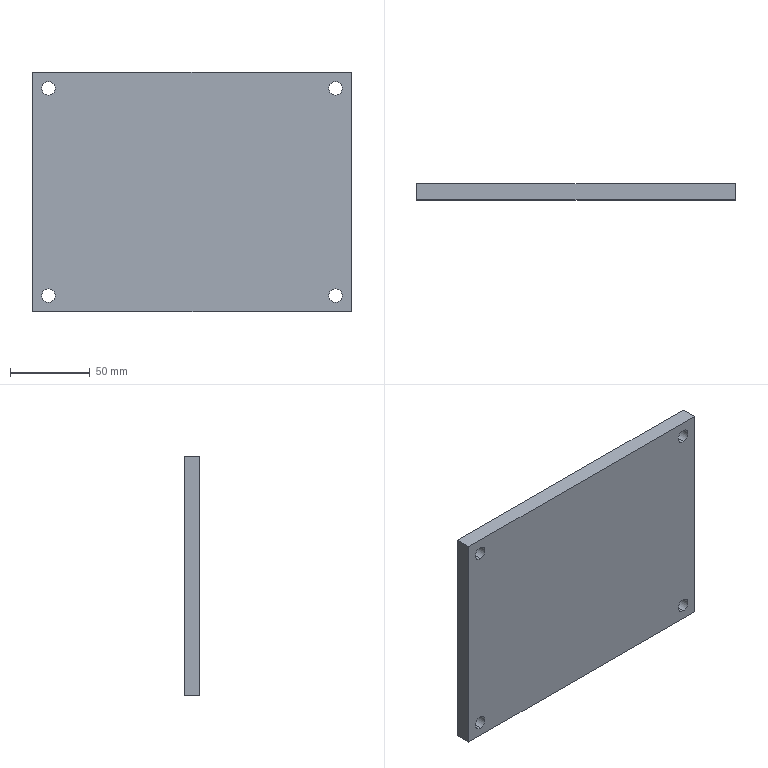Part | 1 solid | 14 faces | box 200 x 10 x 150 mm | volume 297730 mm3 | cylinder 8 | plane 6 | commonest cylinder face diameters 8.5 x8
STEP:
#1=CARTESIAN_POINT('',(-90.,10.,69.25));
#2=VERTEX_POINT('',#1);
#3=CARTESIAN_POINT('',(-90.,10.,60.75));
#4=VERTEX_POINT('',#3);
#5=CARTESIAN_POINT('',(-90.,10.,65.));
#6=DIRECTION('',(0.,-1.,0.));
#7=DIRECTION('',(0.,0.,-1.));
#8=AXIS2_PLACEMENT_3D('',#5,#6,#7);
#9=CIRCLE('',#8,4.25);
#10=EDGE_CURVE('',#2,#4,#9,.T.);
#11=ORIENTED_EDGE('',*,*,#10,.F.);
#12=CARTESIAN_POINT('',(-90.,0.,69.25));
#13=VERTEX_POINT('',#12);
#14=CARTESIAN_POINT('',(-90.,0.,69.25));
#15=DIRECTION('',(0.,-1.,0.));
#16=VECTOR('',#15,1000.);
#17=LINE('',#14,#16);
#18=EDGE_CURVE('',#2,#13,#17,.T.);
#19=ORIENTED_EDGE('',*,*,#18,.T.);
#20=CARTESIAN_POINT('',(-90.,0.,60.75));
#21=VERTEX_POINT('',#20);
#22=CARTESIAN_POINT('',(-90.,0.,65.));
#23=DIRECTION('',(0.,-1.,0.));
#24=DIRECTION('',(0.,0.,-1.));
#25=AXIS2_PLACEMENT_3D('',#22,#23,#24);
#26=CIRCLE('',#25,4.25);
#27=EDGE_CURVE('',#13,#21,#26,.T.);
#28=ORIENTED_EDGE('',*,*,#27,.T.);
#29=CARTESIAN_POINT('',(-90.,0.,60.75));
#30=DIRECTION('',(0.,-1.,0.));
#31=VECTOR('',#30,1000.);
#32=LINE('',#29,#31);
#33=EDGE_CURVE('',#4,#21,#32,.T.);
#34=ORIENTED_EDGE('',*,*,#33,.F.);
#35=EDGE_LOOP('',(#11,#19,#28,#34));
#36=FACE_OUTER_BOUND('',#35,.T.);
#37=CARTESIAN_POINT('',(-90.,0.,65.));
#38=DIRECTION('',(0.,-1.,0.));
#39=DIRECTION('',(0.,0.,-1.));
#40=AXIS2_PLACEMENT_3D('',#37,#38,#39);
#41=CYLINDRICAL_SURFACE('',#40,4.25);
#42=ADVANCED_FACE('',(#36),#41,.F.);
#43=CARTESIAN_POINT('',(-90.,10.,-60.75));
#44=VERTEX_POINT('',#43);
#45=CARTESIAN_POINT('',(-90.,10.,-69.25));
#46=VERTEX_POINT('',#45);
#47=CARTESIAN_POINT('',(-90.,10.,-65.));
#48=DIRECTION('',(0.,-1.,0.));
#49=DIRECTION('',(0.,0.,-1.));
#50=AXIS2_PLACEMENT_3D('',#47,#48,#49);
#51=CIRCLE('',#50,4.25);
#52=EDGE_CURVE('',#44,#46,#51,.T.);
#53=ORIENTED_EDGE('',*,*,#52,.F.);
#54=CARTESIAN_POINT('',(-90.,0.,-60.75));
#55=VERTEX_POINT('',#54);
#56=CARTESIAN_POINT('',(-90.,0.,-60.75));
#57=DIRECTION('',(0.,-1.,0.));
#58=VECTOR('',#57,1000.);
#59=LINE('',#56,#58);
#60=EDGE_CURVE('',#44,#55,#59,.T.);
#61=ORIENTED_EDGE('',*,*,#60,.T.);
#62=CARTESIAN_POINT('',(-90.,0.,-69.25));
#63=VERTEX_POINT('',#62);
#64=CARTESIAN_POINT('',(-90.,0.,-65.));
#65=DIRECTION('',(0.,-1.,0.));
#66=DIRECTION('',(0.,0.,-1.));
#67=AXIS2_PLACEMENT_3D('',#64,#65,#66);
#68=CIRCLE('',#67,4.25);
#69=EDGE_CURVE('',#55,#63,#68,.T.);
#70=ORIENTED_EDGE('',*,*,#69,.T.);
#71=CARTESIAN_POINT('',(-90.,0.,-69.25));
#72=DIRECTION('',(0.,-1.,0.));
#73=VECTOR('',#72,1000.);
#74=LINE('',#71,#73);
#75=EDGE_CURVE('',#46,#63,#74,.T.);
#76=ORIENTED_EDGE('',*,*,#75,.F.);
#77=EDGE_LOOP('',(#53,#61,#70,#76));
#78=FACE_OUTER_BOUND('',#77,.T.);
#79=CARTESIAN_POINT('',(-90.,0.,-65.));
#80=DIRECTION('',(0.,-1.,0.));
#81=DIRECTION('',(0.,0.,-1.));
#82=AXIS2_PLACEMENT_3D('',#79,#80,#81);
#83=CYLINDRICAL_SURFACE('',#82,4.25);
#84=ADVANCED_FACE('',(#78),#83,.F.);
#85=CARTESIAN_POINT('',(90.,10.,-60.75));
#86=VERTEX_POINT('',#85);
#87=CARTESIAN_POINT('',(90.,10.,-69.25));
#88=VERTEX_POINT('',#87);
#89=CARTESIAN_POINT('',(90.,10.,-65.));
#90=DIRECTION('',(0.,-1.,0.));
#91=DIRECTION('',(0.,0.,-1.));
#92=AXIS2_PLACEMENT_3D('',#89,#90,#91);
#93=CIRCLE('',#92,4.25);
#94=EDGE_CURVE('',#86,#88,#93,.T.);
#95=ORIENTED_EDGE('',*,*,#94,.F.);
#96=CARTESIAN_POINT('',(90.,0.,-60.75));
#97=VERTEX_POINT('',#96);
#98=CARTESIAN_POINT('',(90.,0.,-60.75));
#99=DIRECTION('',(0.,-1.,0.));
#100=VECTOR('',#99,1000.);
#101=LINE('',#98,#100);
#102=EDGE_CURVE('',#86,#97,#101,.T.);
#103=ORIENTED_EDGE('',*,*,#102,.T.);
#104=CARTESIAN_POINT('',(90.,0.,-69.25));
#105=VERTEX_POINT('',#104);
#106=CARTESIAN_POINT('',(90.,0.,-65.));
#107=DIRECTION('',(0.,-1.,0.));
#108=DIRECTION('',(0.,0.,-1.));
#109=AXIS2_PLACEMENT_3D('',#106,#107,#108);
#110=CIRCLE('',#109,4.25);
#111=EDGE_CURVE('',#97,#105,#110,.T.);
#112=ORIENTED_EDGE('',*,*,#111,.T.);
#113=CARTESIAN_POINT('',(90.,0.,-69.25));
#114=DIRECTION('',(0.,-1.,0.));
#115=VECTOR('',#114,1000.);
#116=LINE('',#113,#115);
#117=EDGE_CURVE('',#88,#105,#116,.T.);
#118=ORIENTED_EDGE('',*,*,#117,.F.);
#119=EDGE_LOOP('',(#95,#103,#112,#118));
#120=FACE_OUTER_BOUND('',#119,.T.);
#121=CARTESIAN_POINT('',(90.,0.,-65.));
#122=DIRECTION('',(0.,-1.,0.));
#123=DIRECTION('',(0.,0.,-1.));
#124=AXIS2_PLACEMENT_3D('',#121,#122,#123);
#125=CYLINDRICAL_SURFACE('',#124,4.25);
#126=ADVANCED_FACE('',(#120),#125,.F.);
#127=CARTESIAN_POINT('',(90.,10.,69.25));
#128=VERTEX_POINT('',#127);
#129=CARTESIAN_POINT('',(90.,10.,60.75));
#130=VERTEX_POINT('',#129);
#131=CARTESIAN_POINT('',(90.,10.,65.));
#132=DIRECTION('',(0.,-1.,0.));
#133=DIRECTION('',(0.,0.,-1.));
#134=AXIS2_PLACEMENT_3D('',#131,#132,#133);
#135=CIRCLE('',#134,4.25);
#136=EDGE_CURVE('',#128,#130,#135,.T.);
#137=ORIENTED_EDGE('',*,*,#136,.F.);
#138=CARTESIAN_POINT('',(90.,0.,69.25));
#139=VERTEX_POINT('',#138);
#140=CARTESIAN_POINT('',(90.,0.,69.25));
#141=DIRECTION('',(0.,-1.,0.));
#142=VECTOR('',#141,1000.);
#143=LINE('',#140,#142);
#144=EDGE_CURVE('',#128,#139,#143,.T.);
#145=ORIENTED_EDGE('',*,*,#144,.T.);
#146=CARTESIAN_POINT('',(90.,0.,60.75));
#147=VERTEX_POINT('',#146);
#148=CARTESIAN_POINT('',(90.,0.,65.));
#149=DIRECTION('',(0.,-1.,0.));
#150=DIRECTION('',(0.,0.,-1.));
#151=AXIS2_PLACEMENT_3D('',#148,#149,#150);
#152=CIRCLE('',#151,4.25);
#153=EDGE_CURVE('',#139,#147,#152,.T.);
#154=ORIENTED_EDGE('',*,*,#153,.T.);
#155=CARTESIAN_POINT('',(90.,0.,60.75));
#156=DIRECTION('',(0.,-1.,0.));
#157=VECTOR('',#156,1000.);
#158=LINE('',#155,#157);
#159=EDGE_CURVE('',#130,#147,#158,.T.);
#160=ORIENTED_EDGE('',*,*,#159,.F.);
#161=EDGE_LOOP('',(#137,#145,#154,#160));
#162=FACE_OUTER_BOUND('',#161,.T.);
#163=CARTESIAN_POINT('',(90.,0.,65.));
#164=DIRECTION('',(0.,-1.,0.));
#165=DIRECTION('',(0.,0.,-1.));
#166=AXIS2_PLACEMENT_3D('',#163,#164,#165);
#167=CYLINDRICAL_SURFACE('',#166,4.25);
#168=ADVANCED_FACE('',(#162),#167,.F.);
#169=CARTESIAN_POINT('',(100.,0.,75.));
#170=VERTEX_POINT('',#169);
#171=CARTESIAN_POINT('',(100.,0.,-75.));
#172=VERTEX_POINT('',#171);
#173=CARTESIAN_POINT('',(100.,0.,-75.));
#174=DIRECTION('',(0.,0.,-1.));
#175=VECTOR('',#174,1000.);
#176=LINE('',#173,#175);
#177=EDGE_CURVE('',#170,#172,#176,.T.);
#178=ORIENTED_EDGE('',*,*,#177,.T.);
#179=CARTESIAN_POINT('',(100.,10.,-75.));
#180=VERTEX_POINT('',#179);
#181=CARTESIAN_POINT('',(100.,10.,-75.));
#182=DIRECTION('',(0.,-1.,0.));
#183=VECTOR('',#182,1000.);
#184=LINE('',#181,#183);
#185=EDGE_CURVE('',#180,#172,#184,.T.);
#186=ORIENTED_EDGE('',*,*,#185,.F.);
#187=CARTESIAN_POINT('',(100.,10.,75.));
#188=VERTEX_POINT('',#187);
#189=CARTESIAN_POINT('',(100.,10.,-75.));
#190=DIRECTION('',(0.,0.,-1.));
#191=VECTOR('',#190,1000.);
#192=LINE('',#189,#191);
#193=EDGE_CURVE('',#188,#180,#192,.T.);
#194=ORIENTED_EDGE('',*,*,#193,.F.);
#195=CARTESIAN_POINT('',(100.,10.,75.));
#196=DIRECTION('',(0.,-1.,0.));
#197=VECTOR('',#196,1000.);
#198=LINE('',#195,#197);
#199=EDGE_CURVE('',#188,#170,#198,.T.);
#200=ORIENTED_EDGE('',*,*,#199,.T.);
#201=EDGE_LOOP('',(#178,#186,#194,#200));
#202=FACE_OUTER_BOUND('',#201,.T.);
#203=CARTESIAN_POINT('',(100.,10.,-75.));
#204=DIRECTION('',(-1.,0.,0.));
#205=DIRECTION('',(0.,0.,1.));
#206=AXIS2_PLACEMENT_3D('',#203,#204,#205);
#207=PLANE('',#206);
#208=ADVANCED_FACE('',(#202),#207,.F.);
#209=CARTESIAN_POINT('',(-100.,0.,-75.));
#210=VERTEX_POINT('',#209);
#211=CARTESIAN_POINT('',(-100.,0.,-75.));
#212=DIRECTION('',(-1.,0.,0.));
#213=VECTOR('',#212,1000.);
#214=LINE('',#211,#213);
#215=EDGE_CURVE('',#172,#210,#214,.T.);
#216=ORIENTED_EDGE('',*,*,#215,.T.);
#217=CARTESIAN_POINT('',(-100.,10.,-75.));
#218=VERTEX_POINT('',#217);
#219=CARTESIAN_POINT('',(-100.,10.,-75.));
#220=DIRECTION('',(0.,-1.,0.));
#221=VECTOR('',#220,1000.);
#222=LINE('',#219,#221);
#223=EDGE_CURVE('',#218,#210,#222,.T.);
#224=ORIENTED_EDGE('',*,*,#223,.F.);
#225=CARTESIAN_POINT('',(-100.,10.,-75.));
#226=DIRECTION('',(-1.,0.,0.));
#227=VECTOR('',#226,1000.);
#228=LINE('',#225,#227);
#229=EDGE_CURVE('',#180,#218,#228,.T.);
#230=ORIENTED_EDGE('',*,*,#229,.F.);
#231=ORIENTED_EDGE('',*,*,#185,.T.);
#232=EDGE_LOOP('',(#216,#224,#230,#231));
#233=FACE_OUTER_BOUND('',#232,.T.);
#234=CARTESIAN_POINT('',(-100.,10.,-75.));
#235=DIRECTION('',(0.,0.,1.));
#236=DIRECTION('',(1.,0.,0.));
#237=AXIS2_PLACEMENT_3D('',#234,#235,#236);
#238=PLANE('',#237);
#239=ADVANCED_FACE('',(#233),#238,.F.);
#240=CARTESIAN_POINT('',(-100.,0.,75.));
#241=VERTEX_POINT('',#240);
#242=CARTESIAN_POINT('',(-100.,0.,-75.));
#243=DIRECTION('',(0.,0.,1.));
#244=VECTOR('',#243,1000.);
#245=LINE('',#242,#244);
#246=EDGE_CURVE('',#210,#241,#245,.T.);
#247=ORIENTED_EDGE('',*,*,#246,.T.);
#248=CARTESIAN_POINT('',(-100.,10.,75.));
#249=VERTEX_POINT('',#248);
#250=CARTESIAN_POINT('',(-100.,10.,75.));
#251=DIRECTION('',(0.,-1.,0.));
#252=VECTOR('',#251,1000.);
#253=LINE('',#250,#252);
#254=EDGE_CURVE('',#249,#241,#253,.T.);
#255=ORIENTED_EDGE('',*,*,#254,.F.);
#256=CARTESIAN_POINT('',(-100.,10.,-75.));
#257=DIRECTION('',(0.,0.,1.));
#258=VECTOR('',#257,1000.);
#259=LINE('',#256,#258);
#260=EDGE_CURVE('',#218,#249,#259,.T.);
#261=ORIENTED_EDGE('',*,*,#260,.F.);
#262=ORIENTED_EDGE('',*,*,#223,.T.);
#263=EDGE_LOOP('',(#247,#255,#261,#262));
#264=FACE_OUTER_BOUND('',#263,.T.);
#265=CARTESIAN_POINT('',(-100.,10.,-75.));
#266=DIRECTION('',(1.,0.,0.));
#267=DIRECTION('',(0.,0.,-1.));
#268=AXIS2_PLACEMENT_3D('',#265,#266,#267);
#269=PLANE('',#268);
#270=ADVANCED_FACE('',(#264),#269,.F.);
#271=CARTESIAN_POINT('',(-100.,0.,75.));
#272=DIRECTION('',(1.,0.,0.));
#273=VECTOR('',#272,1000.);
#274=LINE('',#271,#273);
#275=EDGE_CURVE('',#241,#170,#274,.T.);
#276=ORIENTED_EDGE('',*,*,#275,.T.);
#277=ORIENTED_EDGE('',*,*,#199,.F.);
#278=CARTESIAN_POINT('',(-100.,10.,75.));
#279=DIRECTION('',(1.,0.,0.));
#280=VECTOR('',#279,1000.);
#281=LINE('',#278,#280);
#282=EDGE_CURVE('',#249,#188,#281,.T.);
#283=ORIENTED_EDGE('',*,*,#282,.F.);
#284=ORIENTED_EDGE('',*,*,#254,.T.);
#285=EDGE_LOOP('',(#276,#277,#283,#284));
#286=FACE_OUTER_BOUND('',#285,.T.);
#287=CARTESIAN_POINT('',(-100.,10.,75.));
#288=DIRECTION('',(0.,0.,-1.));
#289=DIRECTION('',(-1.,0.,0.));
#290=AXIS2_PLACEMENT_3D('',#287,#288,#289);
#291=PLANE('',#290);
#292=ADVANCED_FACE('',(#286),#291,.F.);
#293=CARTESIAN_POINT('',(-90.,10.,65.));
#294=DIRECTION('',(0.,-1.,0.));
#295=DIRECTION('',(0.,0.,-1.));
#296=AXIS2_PLACEMENT_3D('',#293,#294,#295);
#297=CIRCLE('',#296,4.25);
#298=EDGE_CURVE('',#4,#2,#297,.T.);
#299=ORIENTED_EDGE('',*,*,#298,.T.);
#300=ORIENTED_EDGE('',*,*,#10,.T.);
#301=EDGE_LOOP('',(#299,#300));
#302=FACE_BOUND('',#301,.T.);
#303=CARTESIAN_POINT('',(-90.,10.,-65.));
#304=DIRECTION('',(0.,-1.,0.));
#305=DIRECTION('',(0.,0.,-1.));
#306=AXIS2_PLACEMENT_3D('',#303,#304,#305);
#307=CIRCLE('',#306,4.25);
#308=EDGE_CURVE('',#46,#44,#307,.T.);
#309=ORIENTED_EDGE('',*,*,#308,.T.);
#310=ORIENTED_EDGE('',*,*,#52,.T.);
#311=EDGE_LOOP('',(#309,#310));
#312=FACE_BOUND('',#311,.T.);
#313=CARTESIAN_POINT('',(90.,10.,-65.));
#314=DIRECTION('',(0.,-1.,0.));
#315=DIRECTION('',(0.,0.,-1.));
#316=AXIS2_PLACEMENT_3D('',#313,#314,#315);
#317=CIRCLE('',#316,4.25);
#318=EDGE_CURVE('',#88,#86,#317,.T.);
#319=ORIENTED_EDGE('',*,*,#318,.T.);
#320=ORIENTED_EDGE('',*,*,#94,.T.);
#321=EDGE_LOOP('',(#319,#320));
#322=FACE_BOUND('',#321,.T.);
#323=CARTESIAN_POINT('',(90.,10.,65.));
#324=DIRECTION('',(0.,-1.,0.));
#325=DIRECTION('',(0.,0.,-1.));
#326=AXIS2_PLACEMENT_3D('',#323,#324,#325);
#327=CIRCLE('',#326,4.25);
#328=EDGE_CURVE('',#130,#128,#327,.T.);
#329=ORIENTED_EDGE('',*,*,#328,.T.);
#330=ORIENTED_EDGE('',*,*,#136,.T.);
#331=EDGE_LOOP('',(#329,#330));
#332=FACE_BOUND('',#331,.T.);
#333=ORIENTED_EDGE('',*,*,#193,.T.);
#334=ORIENTED_EDGE('',*,*,#229,.T.);
#335=ORIENTED_EDGE('',*,*,#260,.T.);
#336=ORIENTED_EDGE('',*,*,#282,.T.);
#337=EDGE_LOOP('',(#333,#334,#335,#336));
#338=FACE_OUTER_BOUND('',#337,.T.);
#339=CARTESIAN_POINT('',(0.,10.,0.));
#340=DIRECTION('',(0.,1.,0.));
#341=DIRECTION('',(0.,0.,1.));
#342=AXIS2_PLACEMENT_3D('',#339,#340,#341);
#343=PLANE('',#342);
#344=ADVANCED_FACE('',(#302,#312,#322,#332,#338),#343,.T.);
#345=CARTESIAN_POINT('',(-90.,0.,65.));
#346=DIRECTION('',(0.,-1.,0.));
#347=DIRECTION('',(0.,0.,-1.));
#348=AXIS2_PLACEMENT_3D('',#345,#346,#347);
#349=CIRCLE('',#348,4.25);
#350=EDGE_CURVE('',#21,#13,#349,.T.);
#351=ORIENTED_EDGE('',*,*,#350,.F.);
#352=ORIENTED_EDGE('',*,*,#27,.F.);
#353=EDGE_LOOP('',(#351,#352));
#354=FACE_BOUND('',#353,.T.);
#355=CARTESIAN_POINT('',(-90.,0.,-65.));
#356=DIRECTION('',(0.,-1.,0.));
#357=DIRECTION('',(0.,0.,-1.));
#358=AXIS2_PLACEMENT_3D('',#355,#356,#357);
#359=CIRCLE('',#358,4.25);
#360=EDGE_CURVE('',#63,#55,#359,.T.);
#361=ORIENTED_EDGE('',*,*,#360,.F.);
#362=ORIENTED_EDGE('',*,*,#69,.F.);
#363=EDGE_LOOP('',(#361,#362));
#364=FACE_BOUND('',#363,.T.);
#365=CARTESIAN_POINT('',(90.,0.,-65.));
#366=DIRECTION('',(0.,-1.,0.));
#367=DIRECTION('',(0.,0.,-1.));
#368=AXIS2_PLACEMENT_3D('',#365,#366,#367);
#369=CIRCLE('',#368,4.25);
#370=EDGE_CURVE('',#105,#97,#369,.T.);
#371=ORIENTED_EDGE('',*,*,#370,.F.);
#372=ORIENTED_EDGE('',*,*,#111,.F.);
#373=EDGE_LOOP('',(#371,#372));
#374=FACE_BOUND('',#373,.T.);
#375=CARTESIAN_POINT('',(90.,0.,65.));
#376=DIRECTION('',(0.,-1.,0.));
#377=DIRECTION('',(0.,0.,-1.));
#378=AXIS2_PLACEMENT_3D('',#375,#376,#377);
#379=CIRCLE('',#378,4.25);
#380=EDGE_CURVE('',#147,#139,#379,.T.);
#381=ORIENTED_EDGE('',*,*,#380,.F.);
#382=ORIENTED_EDGE('',*,*,#153,.F.);
#383=EDGE_LOOP('',(#381,#382));
#384=FACE_BOUND('',#383,.T.);
#385=ORIENTED_EDGE('',*,*,#177,.F.);
#386=ORIENTED_EDGE('',*,*,#275,.F.);
#387=ORIENTED_EDGE('',*,*,#246,.F.);
#388=ORIENTED_EDGE('',*,*,#215,.F.);
#389=EDGE_LOOP('',(#385,#386,#387,#388));
#390=FACE_OUTER_BOUND('',#389,.T.);
#391=CARTESIAN_POINT('',(0.,0.,0.));
#392=DIRECTION('',(0.,1.,0.));
#393=DIRECTION('',(0.,0.,1.));
#394=AXIS2_PLACEMENT_3D('',#391,#392,#393);
#395=PLANE('',#394);
#396=ADVANCED_FACE('',(#354,#364,#374,#384,#390),#395,.F.);
#397=ORIENTED_EDGE('',*,*,#144,.F.);
#398=ORIENTED_EDGE('',*,*,#328,.F.);
#399=ORIENTED_EDGE('',*,*,#159,.T.);
#400=ORIENTED_EDGE('',*,*,#380,.T.);
#401=EDGE_LOOP('',(#397,#398,#399,#400));
#402=FACE_OUTER_BOUND('',#401,.T.);
#403=CARTESIAN_POINT('',(90.,0.,65.));
#404=DIRECTION('',(0.,-1.,0.));
#405=DIRECTION('',(0.,0.,-1.));
#406=AXIS2_PLACEMENT_3D('',#403,#404,#405);
#407=CYLINDRICAL_SURFACE('',#406,4.25);
#408=ADVANCED_FACE('',(#402),#407,.F.);
#409=ORIENTED_EDGE('',*,*,#102,.F.);
#410=ORIENTED_EDGE('',*,*,#318,.F.);
#411=ORIENTED_EDGE('',*,*,#117,.T.);
#412=ORIENTED_EDGE('',*,*,#370,.T.);
#413=EDGE_LOOP('',(#409,#410,#411,#412));
#414=FACE_OUTER_BOUND('',#413,.T.);
#415=CARTESIAN_POINT('',(90.,0.,-65.));
#416=DIRECTION('',(0.,-1.,0.));
#417=DIRECTION('',(0.,0.,-1.));
#418=AXIS2_PLACEMENT_3D('',#415,#416,#417);
#419=CYLINDRICAL_SURFACE('',#418,4.25);
#420=ADVANCED_FACE('',(#414),#419,.F.);
#421=ORIENTED_EDGE('',*,*,#60,.F.);
#422=ORIENTED_EDGE('',*,*,#308,.F.);
#423=ORIENTED_EDGE('',*,*,#75,.T.);
#424=ORIENTED_EDGE('',*,*,#360,.T.);
#425=EDGE_LOOP('',(#421,#422,#423,#424));
#426=FACE_OUTER_BOUND('',#425,.T.);
#427=CARTESIAN_POINT('',(-90.,0.,-65.));
#428=DIRECTION('',(0.,-1.,0.));
#429=DIRECTION('',(0.,0.,-1.));
#430=AXIS2_PLACEMENT_3D('',#427,#428,#429);
#431=CYLINDRICAL_SURFACE('',#430,4.25);
#432=ADVANCED_FACE('',(#426),#431,.F.);
#433=ORIENTED_EDGE('',*,*,#18,.F.);
#434=ORIENTED_EDGE('',*,*,#298,.F.);
#435=ORIENTED_EDGE('',*,*,#33,.T.);
#436=ORIENTED_EDGE('',*,*,#350,.T.);
#437=EDGE_LOOP('',(#433,#434,#435,#436));
#438=FACE_OUTER_BOUND('',#437,.T.);
#439=CARTESIAN_POINT('',(-90.,0.,65.));
#440=DIRECTION('',(0.,-1.,0.));
#441=DIRECTION('',(0.,0.,-1.));
#442=AXIS2_PLACEMENT_3D('',#439,#440,#441);
#443=CYLINDRICAL_SURFACE('',#442,4.25);
#444=ADVANCED_FACE('',(#438),#443,.F.);
#445=CLOSED_SHELL('',(#42,#84,#126,#168,#208,#239,#270,#292,#344,#396,#408,#420,#432,#444));
#446=MANIFOLD_SOLID_BREP('',#445);
#447=CARTESIAN_POINT('',(0.,0.,0.));
#448=DIRECTION('',(0.,0.,1.));
#449=DIRECTION('',(1.,0.,0.));
#450=AXIS2_PLACEMENT_3D('',#447,#448,#449);
#451=(LENGTH_UNIT()NAMED_UNIT(*)SI_UNIT(.MILLI.,.METRE.));
#452=UNCERTAINTY_MEASURE_WITH_UNIT(LENGTH_MEASURE(0.00001),#451,'','');
#453=(NAMED_UNIT(*)PLANE_ANGLE_UNIT()SI_UNIT($,.RADIAN.));
#454=(NAMED_UNIT(*)SI_UNIT($,.STERADIAN.)SOLID_ANGLE_UNIT());
#455=(GEOMETRIC_REPRESENTATION_CONTEXT(3)GLOBAL_UNCERTAINTY_ASSIGNED_CONTEXT((#452))GLOBAL_UNIT_ASSIGNED_CONTEXT((#451,#453,#454))REPRESENTATION_CONTEXT('',''));
#456=ADVANCED_BREP_SHAPE_REPRESENTATION('',(#446,#450),#455);